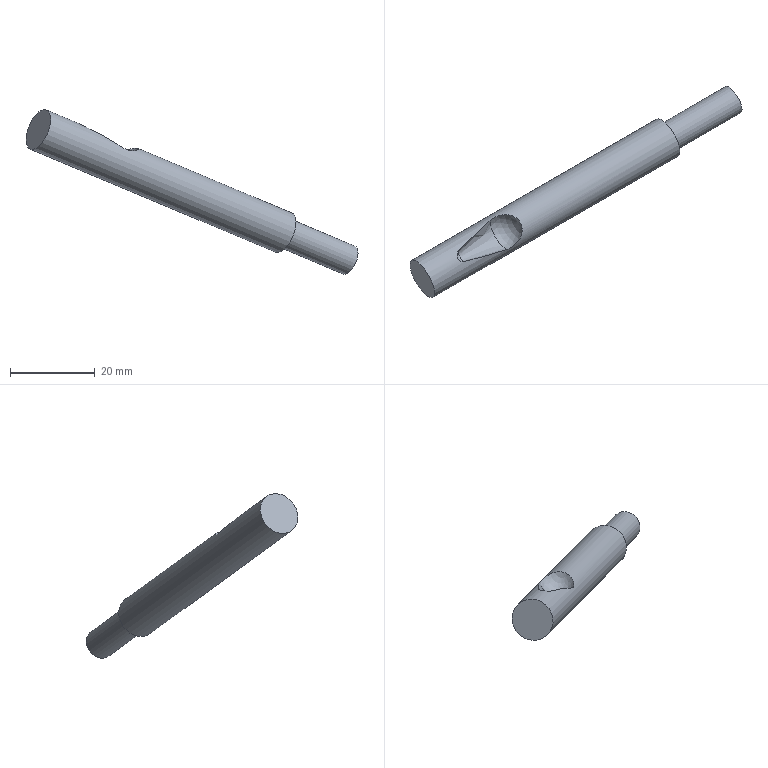Part | NX | features solid 2 | 1 solid | 8 faces | box 78.211 x 49.834 x 38.816 mm | volume 6081 mm3 | plane 3 | cylinder 2 | sphere 2 | cone 1 | commonest cylinder face diameters 7.1 x1 10 x1
STEP:
#1=CARTESIAN_POINT('',(-234.244,-154.892,-18.229));
#2=VERTEX_POINT('',#1);
#3=CARTESIAN_POINT('',(-244.142,-157.737,-12.796));
#4=VERTEX_POINT('',#3);
#5=CARTESIAN_POINT('',(-234.244,-154.892,-18.229));
#6=CARTESIAN_POINT('',(-237.369,-155.928,-16.16));
#7=CARTESIAN_POINT('',(-240.694,-156.832,-14.347));
#8=CARTESIAN_POINT('',(-244.142,-157.737,-12.796));
#9=B_SPLINE_CURVE_WITH_KNOTS('',3,(#5,#6,#7,#8),.UNSPECIFIED.,.F.,.F.,(4,4),(0.000000208,0.01165),.UNSPECIFIED.);
#10=EDGE_CURVE('',#2,#4,#9,.T.);
#11=ORIENTED_EDGE('',*,*,#10,.T.);
#12=CARTESIAN_POINT('',(-245.579,-155.248,-12.796));
#13=VERTEX_POINT('',#12);
#14=CARTESIAN_POINT('',(-244.142,-157.737,-12.796));
#15=CARTESIAN_POINT('',(-244.733,-157.892,-12.53));
#16=CARTESIAN_POINT('',(-246.055,-157.184,-11.896));
#17=CARTESIAN_POINT('',(-246.008,-155.682,-12.53));
#18=CARTESIAN_POINT('',(-245.579,-155.248,-12.796));
#19=B_SPLINE_CURVE_WITH_KNOTS('',3,(#14,#15,#16,#17,#18),.UNSPECIFIED.,.F.,.F.,(4,1,4),(0.000000204,0.001971,0.003941),.UNSPECIFIED.);
#20=EDGE_CURVE('',#4,#13,#19,.T.);
#21=ORIENTED_EDGE('',*,*,#20,.T.);
#22=CARTESIAN_POINT('',(-238.166,-148.099,-18.229));
#23=VERTEX_POINT('',#22);
#24=CARTESIAN_POINT('',(-245.579,-155.248,-12.796));
#25=CARTESIAN_POINT('',(-243.07,-152.713,-14.348));
#26=CARTESIAN_POINT('',(-240.627,-150.289,-16.159));
#27=CARTESIAN_POINT('',(-238.166,-148.099,-18.229));
#28=B_SPLINE_CURVE_WITH_KNOTS('',3,(#24,#25,#26,#27),.UNSPECIFIED.,.F.,.F.,(4,4),(0.000000207,0.01167),.UNSPECIFIED.);
#29=EDGE_CURVE('',#13,#23,#28,.T.);
#30=ORIENTED_EDGE('',*,*,#29,.T.);
#31=CARTESIAN_POINT('',(-238.166,-148.099,-18.229));
#32=CARTESIAN_POINT('',(-237.724,-147.706,-18.6));
#33=CARTESIAN_POINT('',(-236.586,-147.027,-19.111));
#34=CARTESIAN_POINT('',(-234.506,-146.534,-19.025));
#35=CARTESIAN_POINT('',(-232.464,-146.945,-18.55));
#36=CARTESIAN_POINT('',(-230.892,-148.412,-18.279));
#37=CARTESIAN_POINT('',(-230.389,-150.519,-18.546));
#38=CARTESIAN_POINT('',(-231.058,-152.505,-19.025));
#39=CARTESIAN_POINT('',(-232.519,-154.055,-19.112));
#40=CARTESIAN_POINT('',(-233.682,-154.705,-18.601));
#41=CARTESIAN_POINT('',(-234.244,-154.892,-18.229));
#42=B_SPLINE_CURVE_WITH_KNOTS('',3,(#31,#32,#33,#34,#35,#36,#37,#38,#39,#40,#41),.UNSPECIFIED.,.F.,.F.,(4,1,1,1,1,1,1,1,4),(0.000000205,0.002065,0.00413,0.006195,0.00826,0.01033,0.01239,0.01446,0.01652),.UNSPECIFIED.);
#43=EDGE_CURVE('',#23,#2,#42,.T.);
#44=ORIENTED_EDGE('',*,*,#43,.T.);
#45=EDGE_LOOP('',(#11,#21,#30,#44));
#46=FACE_BOUND('',#45,.T.);
#47=CARTESIAN_POINT('',(-251.611,-166.164,-14.004));
#48=VERTEX_POINT('',#47);
#49=CARTESIAN_POINT('',(-254.111,-161.834,-14.004));
#50=DIRECTION('',(-0.8138,-0.4698,0.342));
#51=DIRECTION('',(0.5,-0.866,0.));
#52=AXIS2_PLACEMENT_3D('',#49,#50,#51);
#53=CIRCLE('',#52,5.);
#54=EDGE_CURVE('',#48,#48,#53,.T.);
#55=ORIENTED_EDGE('',*,*,#54,.F.);
#56=EDGE_LOOP('',(#55));
#57=FACE_BOUND('',#56,.T.);
#58=CARTESIAN_POINT('',(-193.832,-132.805,-38.287));
#59=VERTEX_POINT('',#58);
#60=CARTESIAN_POINT('',(-196.332,-128.475,-38.287));
#61=DIRECTION('',(-0.8138,-0.4698,0.342));
#62=DIRECTION('',(0.5,-0.866,0.));
#63=AXIS2_PLACEMENT_3D('',#60,#61,#62);
#64=CIRCLE('',#63,5.);
#65=EDGE_CURVE('',#59,#59,#64,.T.);
#66=ORIENTED_EDGE('',*,*,#65,.T.);
#67=EDGE_LOOP('',(#66));
#68=FACE_BOUND('',#67,.T.);
#69=CARTESIAN_POINT('',(-254.111,-161.834,-14.004));
#70=DIRECTION('',(0.8138,0.4698,-0.342));
#71=DIRECTION('',(-0.5,0.866,0.));
#72=AXIS2_PLACEMENT_3D('',#69,#70,#71);
#73=CYLINDRICAL_SURFACE('',#72,5.);
#74=ADVANCED_FACE('',(#46,#57,#68),#73,.T.);
#75=ORIENTED_EDGE('',*,*,#54,.T.);
#76=EDGE_LOOP('',(#75));
#77=FACE_BOUND('',#76,.T.);
#78=CARTESIAN_POINT('',(-254.111,-161.834,-14.004));
#79=DIRECTION('',(-0.8138,-0.4698,0.342));
#80=DIRECTION('',(0.5,-0.866,0.));
#81=AXIS2_PLACEMENT_3D('',#78,#79,#80);
#82=PLANE('',#81);
#83=ADVANCED_FACE('',(#77),#82,.T.);
#84=CARTESIAN_POINT('',(-194.557,-131.549,-38.287));
#85=VERTEX_POINT('',#84);
#86=CARTESIAN_POINT('',(-196.332,-128.475,-38.287));
#87=DIRECTION('',(-0.8138,-0.4698,0.342));
#88=DIRECTION('',(0.5,-0.866,0.));
#89=AXIS2_PLACEMENT_3D('',#86,#87,#88);
#90=CIRCLE('',#89,3.55);
#91=EDGE_CURVE('',#85,#85,#90,.T.);
#92=ORIENTED_EDGE('',*,*,#91,.T.);
#93=EDGE_LOOP('',(#92));
#94=FACE_BOUND('',#93,.T.);
#95=ORIENTED_EDGE('',*,*,#65,.F.);
#96=EDGE_LOOP('',(#95));
#97=FACE_BOUND('',#96,.T.);
#98=CARTESIAN_POINT('',(-196.332,-128.475,-38.287));
#99=DIRECTION('',(-0.8138,-0.4698,0.342));
#100=DIRECTION('',(0.5,-0.866,0.));
#101=AXIS2_PLACEMENT_3D('',#98,#99,#100);
#102=PLANE('',#101);
#103=ADVANCED_FACE('',(#94,#97),#102,.F.);
#104=CARTESIAN_POINT('',(-179.095,-122.622,-44.786));
#105=VERTEX_POINT('',#104);
#106=CARTESIAN_POINT('',(-180.87,-119.548,-44.786));
#107=DIRECTION('',(-0.8138,-0.4698,0.342));
#108=DIRECTION('',(0.5,-0.866,0.));
#109=AXIS2_PLACEMENT_3D('',#106,#107,#108);
#110=CIRCLE('',#109,3.55);
#111=EDGE_CURVE('',#105,#105,#110,.T.);
#112=ORIENTED_EDGE('',*,*,#111,.T.);
#113=EDGE_LOOP('',(#112));
#114=FACE_BOUND('',#113,.T.);
#115=ORIENTED_EDGE('',*,*,#91,.F.);
#116=EDGE_LOOP('',(#115));
#117=FACE_BOUND('',#116,.T.);
#118=CARTESIAN_POINT('',(-180.87,-119.548,-44.786));
#119=DIRECTION('',(-0.8138,-0.4698,0.342));
#120=DIRECTION('',(0.5,-0.866,0.));
#121=AXIS2_PLACEMENT_3D('',#118,#119,#120);
#122=CYLINDRICAL_SURFACE('',#121,3.55);
#123=ADVANCED_FACE('',(#114,#117),#122,.T.);
#124=ORIENTED_EDGE('',*,*,#111,.F.);
#125=EDGE_LOOP('',(#124));
#126=FACE_BOUND('',#125,.T.);
#127=CARTESIAN_POINT('',(-180.87,-119.548,-44.786));
#128=DIRECTION('',(-0.8138,-0.4698,0.342));
#129=DIRECTION('',(0.5,-0.866,0.));
#130=AXIS2_PLACEMENT_3D('',#127,#128,#129);
#131=PLANE('',#130);
#132=ADVANCED_FACE('',(#126),#131,.F.);
#133=CARTESIAN_POINT('',(-235.642,-151.171,-16.445));
#134=DIRECTION('',(0.8138,0.4698,-0.342));
#135=DIRECTION('',(-0.5,0.866,0.));
#136=AXIS2_PLACEMENT_3D('',#133,#134,#135);
#137=CIRCLE('',#136,4.357);
#138=EDGE_CURVE('',#2,#23,#137,.T.);
#139=ORIENTED_EDGE('',*,*,#138,.F.);
#140=ORIENTED_EDGE('',*,*,#43,.F.);
#141=EDGE_LOOP('',(#139,#140));
#142=FACE_BOUND('',#141,.T.);
#143=CARTESIAN_POINT('',(-234.727,-150.642,-16.83));
#144=DIRECTION('',(0.8138,0.4698,-0.342));
#145=DIRECTION('',(-0.5,0.866,0.));
#146=AXIS2_PLACEMENT_3D('',#143,#144,#145);
#147=SPHERICAL_SURFACE('',#146,4.5);
#148=ADVANCED_FACE('',(#142),#147,.F.);
#149=CARTESIAN_POINT('',(-244.798,-156.457,-12.597));
#150=DIRECTION('',(0.8138,0.4698,-0.342));
#151=DIRECTION('',(-0.5,0.866,0.));
#152=AXIS2_PLACEMENT_3D('',#149,#150,#151);
#153=CIRCLE('',#152,1.452);
#154=EDGE_CURVE('',#4,#13,#153,.T.);
#155=ORIENTED_EDGE('',*,*,#154,.F.);
#156=ORIENTED_EDGE('',*,*,#10,.F.);
#157=ORIENTED_EDGE('',*,*,#138,.T.);
#158=ORIENTED_EDGE('',*,*,#29,.F.);
#159=EDGE_LOOP('',(#155,#156,#157,#158));
#160=FACE_BOUND('',#159,.T.);
#161=CARTESIAN_POINT('',(-235.642,-151.171,-16.445));
#162=DIRECTION('',(0.8138,0.4698,-0.342));
#163=DIRECTION('',(-0.5,0.866,0.));
#164=AXIS2_PLACEMENT_3D('',#161,#162,#163);
#165=CONICAL_SURFACE('',#164,4.357,0.2527);
#166=ADVANCED_FACE('',(#160),#165,.F.);
#167=ORIENTED_EDGE('',*,*,#154,.T.);
#168=ORIENTED_EDGE('',*,*,#20,.F.);
#169=EDGE_LOOP('',(#167,#168));
#170=FACE_BOUND('',#169,.T.);
#171=CARTESIAN_POINT('',(-244.492,-156.28,-12.726));
#172=DIRECTION('',(0.8138,0.4698,-0.342));
#173=DIRECTION('',(0.5,-0.866,0.));
#174=AXIS2_PLACEMENT_3D('',#171,#172,#173);
#175=SPHERICAL_SURFACE('',#174,1.5);
#176=ADVANCED_FACE('',(#170),#175,.F.);
#177=CLOSED_SHELL('',(#74,#83,#103,#123,#132,#148,#166,#176));
#178=MANIFOLD_SOLID_BREP('',#177);
#179=(LENGTH_UNIT()NAMED_UNIT(*)SI_UNIT(.MILLI.,.METRE.));
#180=UNCERTAINTY_MEASURE_WITH_UNIT(LENGTH_MEASURE(0.0508),#179,'','');
#181=(NAMED_UNIT(*)PLANE_ANGLE_UNIT()SI_UNIT($,.RADIAN.));
#182=(NAMED_UNIT(*)SI_UNIT($,.STERADIAN.)SOLID_ANGLE_UNIT());
#183=(GEOMETRIC_REPRESENTATION_CONTEXT(3)GLOBAL_UNCERTAINTY_ASSIGNED_CONTEXT((#180))GLOBAL_UNIT_ASSIGNED_CONTEXT((#179,#181,#182))REPRESENTATION_CONTEXT('',''));
#184=ADVANCED_BREP_SHAPE_REPRESENTATION('',(#178),#183);